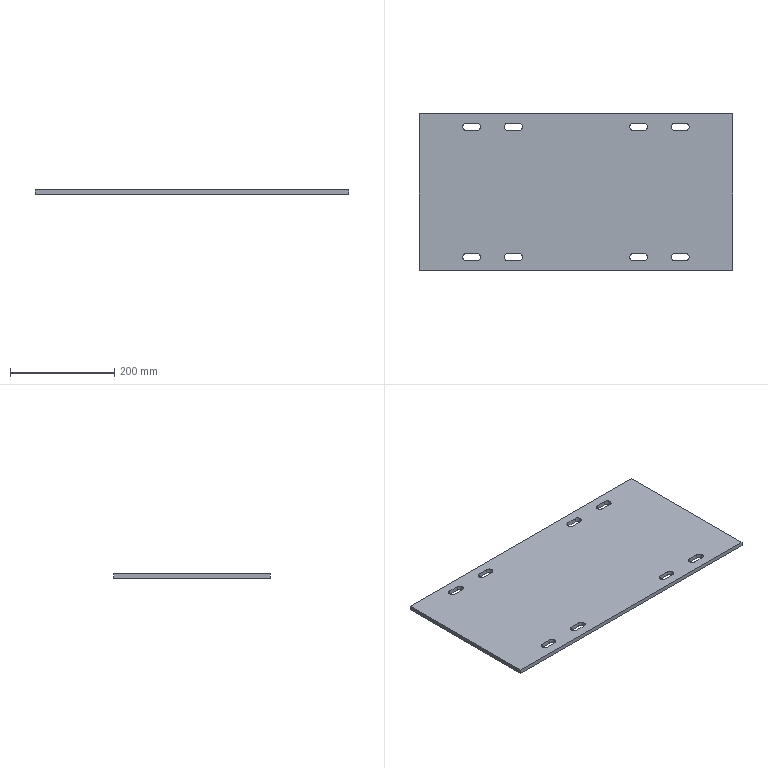Part | STEP file | 02-Base plate | 1 solid | 46 faces | box 600 x 300 x 8 mm | volume 1412228 mm3 | cylinder 24 | plane 22 | commonest cylinder face diameters 14 x24